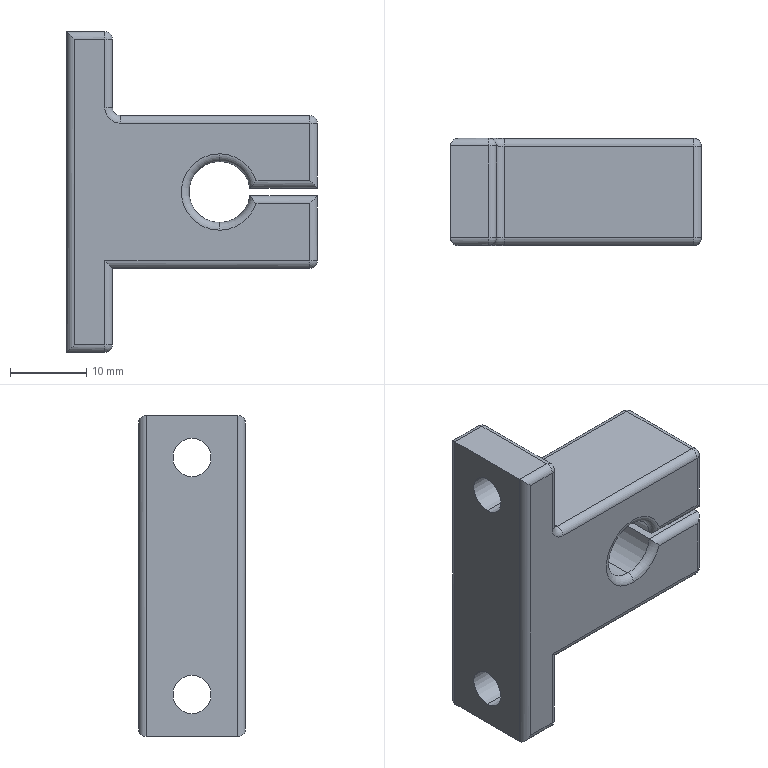Part | STEP file | T-type support 8 | 1 solid | 67 faces | box 32.8 x 14 x 42 mm | volume 9873 mm3 | cylinder 34 | plane 13 | torus 12 | sphere 8 | commonest cylinder face diameters 2 x27 5 x4 8 x3